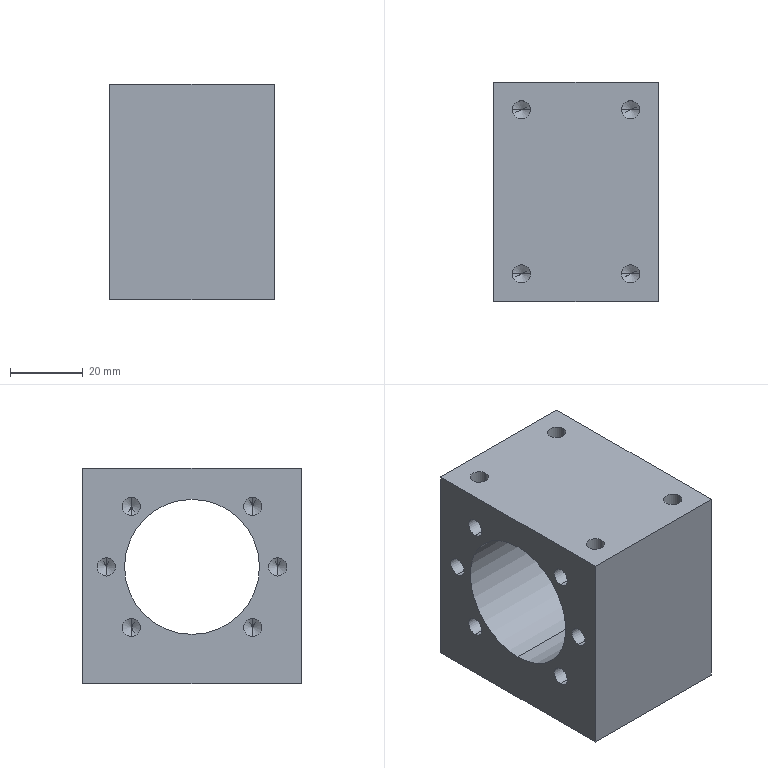Part | STEP file | PN_0025 nut block | 1 solid | 48 faces | box 45 x 60 x 59 mm | volume 107872 mm3 | cylinder 22 | cone 20 | plane 6 | commonest cylinder face diameters 5 x20 37 x2